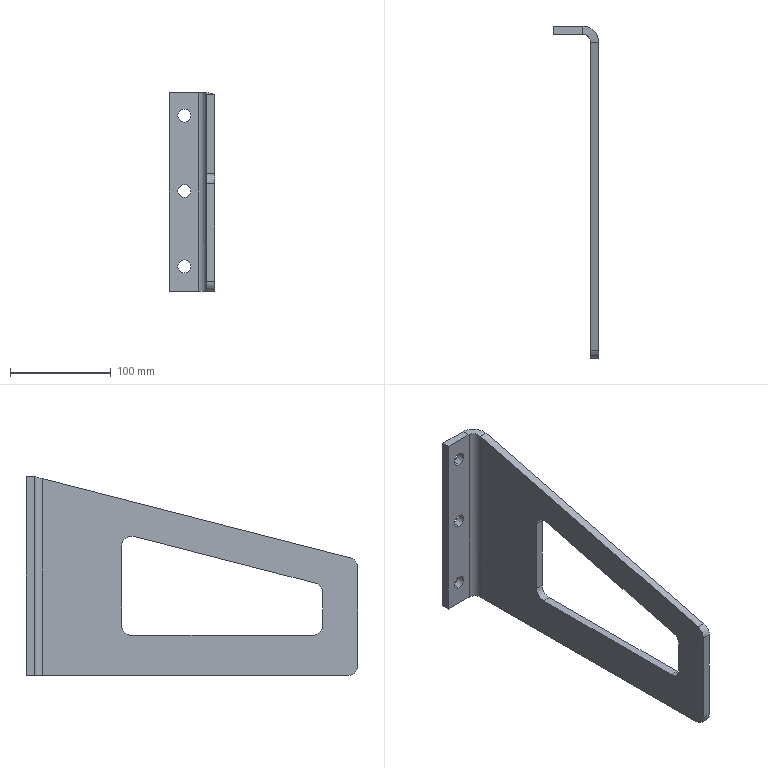Part | SolidWorks | features ICE 2, FlatPattern 1, SMBaseFlange 1, SheetMetal 1 | 1 solid | 30 faces | box 45 x 330 x 197.939 mm | volume 342210 mm3 | plane 15 | cylinder 14 | spline 1 | commonest cylinder face diameters 13 x6 20 x6 16 x1 32 x1
STEP:
#1=CARTESIAN_POINT('',(26.655,269.085,-181.5));
#2=VERTEX_POINT('',#1);
#3=CARTESIAN_POINT('',(26.655,269.085,-168.5));
#4=VERTEX_POINT('',#3);
#5=CARTESIAN_POINT('',(26.655,269.085,-175.));
#6=DIRECTION('',(0.,1.,0.));
#7=DIRECTION('',(0.,0.,1.));
#8=AXIS2_PLACEMENT_3D('',#5,#6,#7);
#9=CIRCLE('',#8,6.5);
#10=EDGE_CURVE('',#2,#4,#9,.T.);
#11=ORIENTED_EDGE('',*,*,#10,.F.);
#12=CARTESIAN_POINT('',(26.655,277.085,-181.5));
#13=VERTEX_POINT('',#12);
#14=CARTESIAN_POINT('',(26.655,-52.915,-181.5));
#15=DIRECTION('',(0.,1.,0.));
#16=VECTOR('',#15,1000.);
#17=LINE('',#14,#16);
#18=EDGE_CURVE('',#2,#13,#17,.T.);
#19=ORIENTED_EDGE('',*,*,#18,.T.);
#20=CARTESIAN_POINT('',(26.655,277.085,-168.5));
#21=VERTEX_POINT('',#20);
#22=CARTESIAN_POINT('',(26.655,277.085,-175.));
#23=DIRECTION('',(0.,1.,0.));
#24=DIRECTION('',(0.,0.,1.));
#25=AXIS2_PLACEMENT_3D('',#22,#23,#24);
#26=CIRCLE('',#25,6.5);
#27=EDGE_CURVE('',#13,#21,#26,.T.);
#28=ORIENTED_EDGE('',*,*,#27,.T.);
#29=CARTESIAN_POINT('',(26.655,-52.915,-168.5));
#30=DIRECTION('',(0.,1.,0.));
#31=VECTOR('',#30,1000.);
#32=LINE('',#29,#31);
#33=EDGE_CURVE('',#4,#21,#32,.T.);
#34=ORIENTED_EDGE('',*,*,#33,.F.);
#35=EDGE_LOOP('',(#11,#19,#28,#34));
#36=FACE_OUTER_BOUND('',#35,.T.);
#37=CARTESIAN_POINT('',(26.655,-52.915,-175.));
#38=DIRECTION('',(0.,1.,0.));
#39=DIRECTION('',(0.,0.,1.));
#40=AXIS2_PLACEMENT_3D('',#37,#38,#39);
#41=CYLINDRICAL_SURFACE('',#40,6.5);
#42=ADVANCED_FACE('',(#36),#41,.F.);
#43=CARTESIAN_POINT('',(26.655,269.085,-106.5));
#44=VERTEX_POINT('',#43);
#45=CARTESIAN_POINT('',(26.655,269.085,-93.5));
#46=VERTEX_POINT('',#45);
#47=CARTESIAN_POINT('',(26.655,269.085,-100.));
#48=DIRECTION('',(0.,1.,0.));
#49=DIRECTION('',(0.,0.,1.));
#50=AXIS2_PLACEMENT_3D('',#47,#48,#49);
#51=CIRCLE('',#50,6.5);
#52=EDGE_CURVE('',#44,#46,#51,.T.);
#53=ORIENTED_EDGE('',*,*,#52,.F.);
#54=CARTESIAN_POINT('',(26.655,277.085,-106.5));
#55=VERTEX_POINT('',#54);
#56=CARTESIAN_POINT('',(26.655,-52.915,-106.5));
#57=DIRECTION('',(0.,1.,0.));
#58=VECTOR('',#57,1000.);
#59=LINE('',#56,#58);
#60=EDGE_CURVE('',#44,#55,#59,.T.);
#61=ORIENTED_EDGE('',*,*,#60,.T.);
#62=CARTESIAN_POINT('',(26.655,277.085,-93.5));
#63=VERTEX_POINT('',#62);
#64=CARTESIAN_POINT('',(26.655,277.085,-100.));
#65=DIRECTION('',(0.,1.,0.));
#66=DIRECTION('',(0.,0.,1.));
#67=AXIS2_PLACEMENT_3D('',#64,#65,#66);
#68=CIRCLE('',#67,6.5);
#69=EDGE_CURVE('',#55,#63,#68,.T.);
#70=ORIENTED_EDGE('',*,*,#69,.T.);
#71=CARTESIAN_POINT('',(26.655,-52.915,-93.5));
#72=DIRECTION('',(0.,1.,0.));
#73=VECTOR('',#72,1000.);
#74=LINE('',#71,#73);
#75=EDGE_CURVE('',#46,#63,#74,.T.);
#76=ORIENTED_EDGE('',*,*,#75,.F.);
#77=EDGE_LOOP('',(#53,#61,#70,#76));
#78=FACE_OUTER_BOUND('',#77,.T.);
#79=CARTESIAN_POINT('',(26.655,-52.915,-100.));
#80=DIRECTION('',(0.,1.,0.));
#81=DIRECTION('',(0.,0.,1.));
#82=AXIS2_PLACEMENT_3D('',#79,#80,#81);
#83=CYLINDRICAL_SURFACE('',#82,6.5);
#84=ADVANCED_FACE('',(#78),#83,.F.);
#85=CARTESIAN_POINT('',(26.655,269.085,-31.5));
#86=VERTEX_POINT('',#85);
#87=CARTESIAN_POINT('',(26.655,269.085,-18.5));
#88=VERTEX_POINT('',#87);
#89=CARTESIAN_POINT('',(26.655,269.085,-25.));
#90=DIRECTION('',(0.,1.,0.));
#91=DIRECTION('',(0.,0.,1.));
#92=AXIS2_PLACEMENT_3D('',#89,#90,#91);
#93=CIRCLE('',#92,6.5);
#94=EDGE_CURVE('',#86,#88,#93,.T.);
#95=ORIENTED_EDGE('',*,*,#94,.F.);
#96=CARTESIAN_POINT('',(26.655,277.085,-31.5));
#97=VERTEX_POINT('',#96);
#98=CARTESIAN_POINT('',(26.655,-52.915,-31.5));
#99=DIRECTION('',(0.,1.,0.));
#100=VECTOR('',#99,1000.);
#101=LINE('',#98,#100);
#102=EDGE_CURVE('',#86,#97,#101,.T.);
#103=ORIENTED_EDGE('',*,*,#102,.T.);
#104=CARTESIAN_POINT('',(26.655,277.085,-18.5));
#105=VERTEX_POINT('',#104);
#106=CARTESIAN_POINT('',(26.655,277.085,-25.));
#107=DIRECTION('',(0.,1.,0.));
#108=DIRECTION('',(0.,0.,1.));
#109=AXIS2_PLACEMENT_3D('',#106,#107,#108);
#110=CIRCLE('',#109,6.5);
#111=EDGE_CURVE('',#97,#105,#110,.T.);
#112=ORIENTED_EDGE('',*,*,#111,.T.);
#113=CARTESIAN_POINT('',(26.655,-52.915,-18.5));
#114=DIRECTION('',(0.,1.,0.));
#115=VECTOR('',#114,1000.);
#116=LINE('',#113,#115);
#117=EDGE_CURVE('',#88,#105,#116,.T.);
#118=ORIENTED_EDGE('',*,*,#117,.F.);
#119=EDGE_LOOP('',(#95,#103,#112,#118));
#120=FACE_OUTER_BOUND('',#119,.T.);
#121=CARTESIAN_POINT('',(26.655,-52.915,-25.));
#122=DIRECTION('',(0.,1.,0.));
#123=DIRECTION('',(0.,0.,1.));
#124=AXIS2_PLACEMENT_3D('',#121,#122,#123);
#125=CYLINDRICAL_SURFACE('',#124,6.5);
#126=ADVANCED_FACE('',(#120),#125,.F.);
#127=CARTESIAN_POINT('',(56.655,-7.915,-160.));
#128=VERTEX_POINT('',#127);
#129=CARTESIAN_POINT('',(56.655,172.085,-160.));
#130=VERTEX_POINT('',#129);
#131=CARTESIAN_POINT('',(56.655,-52.915,-160.));
#132=DIRECTION('',(0.,1.,0.));
#133=VECTOR('',#132,1000.);
#134=LINE('',#131,#133);
#135=EDGE_CURVE('',#128,#130,#134,.T.);
#136=ORIENTED_EDGE('',*,*,#135,.F.);
#137=CARTESIAN_POINT('',(56.655,-17.915,-150.));
#138=VERTEX_POINT('',#137);
#139=CARTESIAN_POINT('',(56.655,-7.915,-150.));
#140=DIRECTION('',(1.,0.,0.));
#141=DIRECTION('',(0.,0.,-1.));
#142=AXIS2_PLACEMENT_3D('',#139,#140,#141);
#143=CIRCLE('',#142,10.);
#144=EDGE_CURVE('',#138,#128,#143,.T.);
#145=ORIENTED_EDGE('',*,*,#144,.F.);
#146=CARTESIAN_POINT('',(56.655,-17.915,-117.751));
#147=VERTEX_POINT('',#146);
#148=CARTESIAN_POINT('',(56.655,-17.915,-200.));
#149=DIRECTION('',(0.,0.,-1.));
#150=VECTOR('',#149,1000.);
#151=LINE('',#148,#150);
#152=EDGE_CURVE('',#147,#138,#151,.T.);
#153=ORIENTED_EDGE('',*,*,#152,.F.);
#154=CARTESIAN_POINT('',(56.655,-10.408,-108.067));
#155=VERTEX_POINT('',#154);
#156=CARTESIAN_POINT('',(56.655,-7.915,-117.751));
#157=DIRECTION('',(1.,0.,0.));
#158=DIRECTION('',(0.,0.,-1.));
#159=AXIS2_PLACEMENT_3D('',#156,#157,#158);
#160=CIRCLE('',#159,10.);
#161=EDGE_CURVE('',#155,#147,#160,.T.);
#162=ORIENTED_EDGE('',*,*,#161,.F.);
#163=CARTESIAN_POINT('',(56.655,169.592,-61.717));
#164=VERTEX_POINT('',#163);
#165=CARTESIAN_POINT('',(56.655,-72.472,-124.049));
#166=DIRECTION('',(0.,-0.9684,-0.2494));
#167=VECTOR('',#166,1000.);
#168=LINE('',#165,#167);
#169=EDGE_CURVE('',#164,#155,#168,.T.);
#170=ORIENTED_EDGE('',*,*,#169,.F.);
#171=CARTESIAN_POINT('',(56.655,182.085,-71.401));
#172=VERTEX_POINT('',#171);
#173=CARTESIAN_POINT('',(56.655,172.085,-71.401));
#174=DIRECTION('',(1.,0.,0.));
#175=DIRECTION('',(0.,0.,-1.));
#176=AXIS2_PLACEMENT_3D('',#173,#174,#175);
#177=CIRCLE('',#176,10.);
#178=EDGE_CURVE('',#172,#164,#177,.T.);
#179=ORIENTED_EDGE('',*,*,#178,.F.);
#180=CARTESIAN_POINT('',(56.655,182.085,-150.));
#181=VERTEX_POINT('',#180);
#182=CARTESIAN_POINT('',(56.655,182.085,-200.));
#183=DIRECTION('',(0.,0.,1.));
#184=VECTOR('',#183,1000.);
#185=LINE('',#182,#184);
#186=EDGE_CURVE('',#181,#172,#185,.T.);
#187=ORIENTED_EDGE('',*,*,#186,.F.);
#188=CARTESIAN_POINT('',(56.655,172.085,-150.));
#189=DIRECTION('',(1.,0.,0.));
#190=DIRECTION('',(0.,0.,-1.));
#191=AXIS2_PLACEMENT_3D('',#188,#189,#190);
#192=CIRCLE('',#191,10.);
#193=EDGE_CURVE('',#130,#181,#192,.T.);
#194=ORIENTED_EDGE('',*,*,#193,.F.);
#195=EDGE_LOOP('',(#136,#145,#153,#162,#170,#179,#187,#194));
#196=FACE_BOUND('',#195,.T.);
#197=CARTESIAN_POINT('',(56.655,-45.409,-83.067));
#198=VERTEX_POINT('',#197);
#199=CARTESIAN_POINT('',(56.655,261.085,-4.121));
#200=VERTEX_POINT('',#199);
#201=CARTESIAN_POINT('',(56.655,-45.409,-83.067));
#202=DIRECTION('',(0.,0.9684,0.2494));
#203=VECTOR('',#202,1000.);
#204=LINE('',#201,#203);
#205=EDGE_CURVE('',#198,#200,#204,.T.);
#206=ORIENTED_EDGE('',*,*,#205,.F.);
#207=CARTESIAN_POINT('',(56.655,-52.915,-92.751));
#208=VERTEX_POINT('',#207);
#209=CARTESIAN_POINT('',(56.655,-42.915,-92.751));
#210=DIRECTION('',(-1.,0.,0.));
#211=DIRECTION('',(0.,0.,1.));
#212=AXIS2_PLACEMENT_3D('',#209,#210,#211);
#213=CIRCLE('',#212,10.);
#214=EDGE_CURVE('',#208,#198,#213,.T.);
#215=ORIENTED_EDGE('',*,*,#214,.F.);
#216=CARTESIAN_POINT('',(56.655,-52.915,-190.));
#217=VERTEX_POINT('',#216);
#218=CARTESIAN_POINT('',(56.655,-52.915,-200.));
#219=DIRECTION('',(0.,0.,1.));
#220=VECTOR('',#219,1000.);
#221=LINE('',#218,#220);
#222=EDGE_CURVE('',#217,#208,#221,.T.);
#223=ORIENTED_EDGE('',*,*,#222,.F.);
#224=CARTESIAN_POINT('',(56.655,-42.915,-200.));
#225=VERTEX_POINT('',#224);
#226=CARTESIAN_POINT('',(56.655,-42.915,-190.));
#227=DIRECTION('',(-1.,0.,0.));
#228=DIRECTION('',(0.,0.,-1.));
#229=AXIS2_PLACEMENT_3D('',#226,#227,#228);
#230=CIRCLE('',#229,10.);
#231=EDGE_CURVE('',#225,#217,#230,.T.);
#232=ORIENTED_EDGE('',*,*,#231,.F.);
#233=CARTESIAN_POINT('',(56.655,261.085,-200.));
#234=VERTEX_POINT('',#233);
#235=CARTESIAN_POINT('',(56.655,-52.915,-200.));
#236=DIRECTION('',(0.,1.,0.));
#237=VECTOR('',#236,1000.);
#238=LINE('',#235,#237);
#239=EDGE_CURVE('',#225,#234,#238,.T.);
#240=ORIENTED_EDGE('',*,*,#239,.T.);
#241=CARTESIAN_POINT('',(56.655,261.085,-200.));
#242=DIRECTION('',(0.,0.,1.));
#243=VECTOR('',#242,1000.);
#244=LINE('',#241,#243);
#245=EDGE_CURVE('',#234,#200,#244,.T.);
#246=ORIENTED_EDGE('',*,*,#245,.T.);
#247=EDGE_LOOP('',(#206,#215,#223,#232,#240,#246));
#248=FACE_OUTER_BOUND('',#247,.T.);
#249=CARTESIAN_POINT('',(56.655,-52.915,-200.));
#250=DIRECTION('',(1.,0.,0.));
#251=DIRECTION('',(0.,0.,-1.));
#252=AXIS2_PLACEMENT_3D('',#249,#250,#251);
#253=PLANE('',#252);
#254=ADVANCED_FACE('',(#196,#248),#253,.T.);
#255=CARTESIAN_POINT('',(48.655,-17.915,-150.));
#256=VERTEX_POINT('',#255);
#257=CARTESIAN_POINT('',(48.655,-7.915,-160.));
#258=VERTEX_POINT('',#257);
#259=CARTESIAN_POINT('',(48.655,-7.915,-150.));
#260=DIRECTION('',(1.,0.,0.));
#261=DIRECTION('',(0.,0.,-1.));
#262=AXIS2_PLACEMENT_3D('',#259,#260,#261);
#263=CIRCLE('',#262,10.);
#264=EDGE_CURVE('',#256,#258,#263,.T.);
#265=ORIENTED_EDGE('',*,*,#264,.T.);
#266=CARTESIAN_POINT('',(48.655,172.085,-160.));
#267=VERTEX_POINT('',#266);
#268=CARTESIAN_POINT('',(48.655,-52.915,-160.));
#269=DIRECTION('',(0.,1.,0.));
#270=VECTOR('',#269,1000.);
#271=LINE('',#268,#270);
#272=EDGE_CURVE('',#258,#267,#271,.T.);
#273=ORIENTED_EDGE('',*,*,#272,.T.);
#274=CARTESIAN_POINT('',(48.655,182.085,-150.));
#275=VERTEX_POINT('',#274);
#276=CARTESIAN_POINT('',(48.655,172.085,-150.));
#277=DIRECTION('',(1.,0.,0.));
#278=DIRECTION('',(0.,0.,-1.));
#279=AXIS2_PLACEMENT_3D('',#276,#277,#278);
#280=CIRCLE('',#279,10.);
#281=EDGE_CURVE('',#267,#275,#280,.T.);
#282=ORIENTED_EDGE('',*,*,#281,.T.);
#283=CARTESIAN_POINT('',(48.655,182.085,-71.401));
#284=VERTEX_POINT('',#283);
#285=CARTESIAN_POINT('',(48.655,182.085,-200.));
#286=DIRECTION('',(0.,0.,1.));
#287=VECTOR('',#286,1000.);
#288=LINE('',#285,#287);
#289=EDGE_CURVE('',#275,#284,#288,.T.);
#290=ORIENTED_EDGE('',*,*,#289,.T.);
#291=CARTESIAN_POINT('',(48.655,169.592,-61.717));
#292=VERTEX_POINT('',#291);
#293=CARTESIAN_POINT('',(48.655,172.085,-71.401));
#294=DIRECTION('',(1.,0.,0.));
#295=DIRECTION('',(0.,0.,-1.));
#296=AXIS2_PLACEMENT_3D('',#293,#294,#295);
#297=CIRCLE('',#296,10.);
#298=EDGE_CURVE('',#284,#292,#297,.T.);
#299=ORIENTED_EDGE('',*,*,#298,.T.);
#300=CARTESIAN_POINT('',(48.655,-10.408,-108.067));
#301=VERTEX_POINT('',#300);
#302=CARTESIAN_POINT('',(48.655,-72.472,-124.049));
#303=DIRECTION('',(0.,-0.9684,-0.2494));
#304=VECTOR('',#303,1000.);
#305=LINE('',#302,#304);
#306=EDGE_CURVE('',#292,#301,#305,.T.);
#307=ORIENTED_EDGE('',*,*,#306,.T.);
#308=CARTESIAN_POINT('',(48.655,-17.915,-117.751));
#309=VERTEX_POINT('',#308);
#310=CARTESIAN_POINT('',(48.655,-7.915,-117.751));
#311=DIRECTION('',(1.,0.,0.));
#312=DIRECTION('',(0.,0.,-1.));
#313=AXIS2_PLACEMENT_3D('',#310,#311,#312);
#314=CIRCLE('',#313,10.);
#315=EDGE_CURVE('',#301,#309,#314,.T.);
#316=ORIENTED_EDGE('',*,*,#315,.T.);
#317=CARTESIAN_POINT('',(48.655,-17.915,-200.));
#318=DIRECTION('',(0.,0.,-1.));
#319=VECTOR('',#318,1000.);
#320=LINE('',#317,#319);
#321=EDGE_CURVE('',#309,#256,#320,.T.);
#322=ORIENTED_EDGE('',*,*,#321,.T.);
#323=EDGE_LOOP('',(#265,#273,#282,#290,#299,#307,#316,#322));
#324=FACE_BOUND('',#323,.T.);
#325=CARTESIAN_POINT('',(48.655,-52.915,-92.751));
#326=VERTEX_POINT('',#325);
#327=CARTESIAN_POINT('',(48.655,-45.409,-83.067));
#328=VERTEX_POINT('',#327);
#329=CARTESIAN_POINT('',(48.655,-42.915,-92.751));
#330=DIRECTION('',(-1.,0.,0.));
#331=DIRECTION('',(0.,0.,1.));
#332=AXIS2_PLACEMENT_3D('',#329,#330,#331);
#333=CIRCLE('',#332,10.);
#334=EDGE_CURVE('',#326,#328,#333,.T.);
#335=ORIENTED_EDGE('',*,*,#334,.T.);
#336=CARTESIAN_POINT('',(48.655,261.085,-4.121));
#337=VERTEX_POINT('',#336);
#338=CARTESIAN_POINT('',(48.655,-45.409,-83.067));
#339=DIRECTION('',(0.,0.9684,0.2494));
#340=VECTOR('',#339,1000.);
#341=LINE('',#338,#340);
#342=EDGE_CURVE('',#328,#337,#341,.T.);
#343=ORIENTED_EDGE('',*,*,#342,.T.);
#344=CARTESIAN_POINT('',(48.655,261.085,-200.));
#345=VERTEX_POINT('',#344);
#346=CARTESIAN_POINT('',(48.655,261.085,-200.));
#347=DIRECTION('',(0.,0.,1.));
#348=VECTOR('',#347,1000.);
#349=LINE('',#346,#348);
#350=EDGE_CURVE('',#345,#337,#349,.T.);
#351=ORIENTED_EDGE('',*,*,#350,.F.);
#352=CARTESIAN_POINT('',(48.655,-42.915,-200.));
#353=VERTEX_POINT('',#352);
#354=CARTESIAN_POINT('',(48.655,-52.915,-200.));
#355=DIRECTION('',(0.,1.,0.));
#356=VECTOR('',#355,1000.);
#357=LINE('',#354,#356);
#358=EDGE_CURVE('',#353,#345,#357,.T.);
#359=ORIENTED_EDGE('',*,*,#358,.F.);
#360=CARTESIAN_POINT('',(48.655,-52.915,-190.));
#361=VERTEX_POINT('',#360);
#362=CARTESIAN_POINT('',(48.655,-42.915,-190.));
#363=DIRECTION('',(-1.,0.,0.));
#364=DIRECTION('',(0.,0.,-1.));
#365=AXIS2_PLACEMENT_3D('',#362,#363,#364);
#366=CIRCLE('',#365,10.);
#367=EDGE_CURVE('',#353,#361,#366,.T.);
#368=ORIENTED_EDGE('',*,*,#367,.T.);
#369=CARTESIAN_POINT('',(48.655,-52.915,-200.));
#370=DIRECTION('',(0.,0.,1.));
#371=VECTOR('',#370,1000.);
#372=LINE('',#369,#371);
#373=EDGE_CURVE('',#361,#326,#372,.T.);
#374=ORIENTED_EDGE('',*,*,#373,.T.);
#375=EDGE_LOOP('',(#335,#343,#351,#359,#368,#374));
#376=FACE_OUTER_BOUND('',#375,.T.);
#377=CARTESIAN_POINT('',(48.655,-52.915,-200.));
#378=DIRECTION('',(1.,0.,0.));
#379=DIRECTION('',(0.,0.,-1.));
#380=AXIS2_PLACEMENT_3D('',#377,#378,#379);
#381=PLANE('',#380);
#382=ADVANCED_FACE('',(#324,#376),#381,.F.);
#383=CARTESIAN_POINT('',(26.655,277.085,-175.));
#384=DIRECTION('',(0.,1.,0.));
#385=DIRECTION('',(0.,0.,1.));
#386=AXIS2_PLACEMENT_3D('',#383,#384,#385);
#387=CIRCLE('',#386,6.5);
#388=EDGE_CURVE('',#21,#13,#387,.T.);
#389=ORIENTED_EDGE('',*,*,#388,.F.);
#390=ORIENTED_EDGE('',*,*,#27,.F.);
#391=EDGE_LOOP('',(#389,#390));
#392=FACE_BOUND('',#391,.T.);
#393=CARTESIAN_POINT('',(26.655,277.085,-100.));
#394=DIRECTION('',(0.,1.,0.));
#395=DIRECTION('',(0.,0.,1.));
#396=AXIS2_PLACEMENT_3D('',#393,#394,#395);
#397=CIRCLE('',#396,6.5);
#398=EDGE_CURVE('',#63,#55,#397,.T.);
#399=ORIENTED_EDGE('',*,*,#398,.F.);
#400=ORIENTED_EDGE('',*,*,#69,.F.);
#401=EDGE_LOOP('',(#399,#400));
#402=FACE_BOUND('',#401,.T.);
#403=CARTESIAN_POINT('',(26.655,277.085,-25.));
#404=DIRECTION('',(0.,1.,0.));
#405=DIRECTION('',(0.,0.,1.));
#406=AXIS2_PLACEMENT_3D('',#403,#404,#405);
#407=CIRCLE('',#406,6.5);
#408=EDGE_CURVE('',#105,#97,#407,.T.);
#409=ORIENTED_EDGE('',*,*,#408,.F.);
#410=ORIENTED_EDGE('',*,*,#111,.F.);
#411=EDGE_LOOP('',(#409,#410));
#412=FACE_BOUND('',#411,.T.);
#413=CARTESIAN_POINT('',(11.655,277.085,-200.));
#414=VERTEX_POINT('',#413);
#415=CARTESIAN_POINT('',(11.655,277.085,-2.061));
#416=VERTEX_POINT('',#415);
#417=CARTESIAN_POINT('',(11.655,277.085,-200.));
#418=DIRECTION('',(0.,0.,1.));
#419=VECTOR('',#418,1000.);
#420=LINE('',#417,#419);
#421=EDGE_CURVE('',#414,#416,#420,.T.);
#422=ORIENTED_EDGE('',*,*,#421,.T.);
#423=CARTESIAN_POINT('',(40.655,277.085,-2.061));
#424=VERTEX_POINT('',#423);
#425=CARTESIAN_POINT('',(48.655,277.085,-2.061));
#426=DIRECTION('',(-1.,0.,0.));
#427=VECTOR('',#426,1000.);
#428=LINE('',#425,#427);
#429=EDGE_CURVE('',#424,#416,#428,.T.);
#430=ORIENTED_EDGE('',*,*,#429,.F.);
#431=CARTESIAN_POINT('',(40.655,277.085,-200.));
#432=VERTEX_POINT('',#431);
#433=CARTESIAN_POINT('',(40.655,277.085,-200.));
#434=DIRECTION('',(0.,0.,1.));
#435=VECTOR('',#434,1000.);
#436=LINE('',#433,#435);
#437=EDGE_CURVE('',#432,#424,#436,.T.);
#438=ORIENTED_EDGE('',*,*,#437,.F.);
#439=CARTESIAN_POINT('',(48.655,277.085,-200.));
#440=DIRECTION('',(-1.,0.,0.));
#441=VECTOR('',#440,1000.);
#442=LINE('',#439,#441);
#443=EDGE_CURVE('',#432,#414,#442,.T.);
#444=ORIENTED_EDGE('',*,*,#443,.T.);
#445=EDGE_LOOP('',(#422,#430,#438,#444));
#446=FACE_OUTER_BOUND('',#445,.T.);
#447=CARTESIAN_POINT('',(48.655,277.085,-200.));
#448=DIRECTION('',(0.,1.,0.));
#449=DIRECTION('',(0.,0.,1.));
#450=AXIS2_PLACEMENT_3D('',#447,#448,#449);
#451=PLANE('',#450);
#452=ADVANCED_FACE('',(#392,#402,#412,#446),#451,.T.);
#453=ORIENTED_EDGE('',*,*,#437,.T.);
#454=CARTESIAN_POINT('',(56.655,261.085,-4.121));
#455=CARTESIAN_POINT('',(56.655,270.458,-2.914));
#456=CARTESIAN_POINT('',(50.027,277.085,-2.061));
#457=CARTESIAN_POINT('',(40.655,277.085,-2.061));
#458=(BOUNDED_CURVE()B_SPLINE_CURVE(3,(#454,#455,#456,#457),.UNSPECIFIED.,.F.,.T.)B_SPLINE_CURVE_WITH_KNOTS((4,4),(4.712,6.283),.UNSPECIFIED.)CURVE()GEOMETRIC_REPRESENTATION_ITEM()RATIONAL_B_SPLINE_CURVE((1.,0.8047,0.8047,1.))REPRESENTATION_ITEM(''));
#459=EDGE_CURVE('',#200,#424,#458,.T.);
#460=ORIENTED_EDGE('',*,*,#459,.F.);
#461=ORIENTED_EDGE('',*,*,#245,.F.);
#462=CARTESIAN_POINT('',(40.655,261.085,-200.));
#463=DIRECTION('',(0.,0.,1.));
#464=DIRECTION('',(1.,0.,0.));
#465=AXIS2_PLACEMENT_3D('',#462,#463,#464);
#466=CIRCLE('',#465,16.);
#467=EDGE_CURVE('',#234,#432,#466,.T.);
#468=ORIENTED_EDGE('',*,*,#467,.T.);
#469=EDGE_LOOP('',(#453,#460,#461,#468));
#470=FACE_OUTER_BOUND('',#469,.T.);
#471=CARTESIAN_POINT('',(40.655,261.085,-200.));
#472=DIRECTION('',(0.,0.,1.));
#473=DIRECTION('',(1.,0.,0.));
#474=AXIS2_PLACEMENT_3D('',#471,#472,#473);
#475=CYLINDRICAL_SURFACE('',#474,16.);
#476=ADVANCED_FACE('',(#470),#475,.T.);
#477=CARTESIAN_POINT('',(40.655,269.085,-2.061));
#478=VERTEX_POINT('',#477);
#479=CARTESIAN_POINT('',(48.655,261.085,-4.121));
#480=CARTESIAN_POINT('',(48.655,265.772,-2.914));
#481=CARTESIAN_POINT('',(45.341,269.085,-2.061));
#482=CARTESIAN_POINT('',(40.655,269.085,-2.061));
#483=(BOUNDED_CURVE()B_SPLINE_CURVE(3,(#479,#480,#481,#482),.UNSPECIFIED.,.F.,.T.)B_SPLINE_CURVE_WITH_KNOTS((4,4),(4.712,6.283),.UNSPECIFIED.)CURVE()GEOMETRIC_REPRESENTATION_ITEM()RATIONAL_B_SPLINE_CURVE((1.,0.8047,0.8047,1.))REPRESENTATION_ITEM(''));
#484=EDGE_CURVE('',#337,#478,#483,.T.);
#485=ORIENTED_EDGE('',*,*,#484,.T.);
#486=CARTESIAN_POINT('',(40.655,269.085,-200.));
#487=VERTEX_POINT('',#486);
#488=CARTESIAN_POINT('',(40.655,269.085,-200.));
#489=DIRECTION('',(0.,0.,1.));
#490=VECTOR('',#489,1000.);
#491=LINE('',#488,#490);
#492=EDGE_CURVE('',#487,#478,#491,.T.);
#493=ORIENTED_EDGE('',*,*,#492,.F.);
#494=CARTESIAN_POINT('',(40.655,261.085,-200.));
#495=DIRECTION('',(0.,0.,1.));
#496=DIRECTION('',(-1.,0.,0.));
#497=AXIS2_PLACEMENT_3D('',#494,#495,#496);
#498=CIRCLE('',#497,8.);
#499=EDGE_CURVE('',#345,#487,#498,.T.);
#500=ORIENTED_EDGE('',*,*,#499,.F.);
#501=ORIENTED_EDGE('',*,*,#350,.T.);
#502=EDGE_LOOP('',(#485,#493,#500,#501));
#503=FACE_OUTER_BOUND('',#502,.T.);
#504=CARTESIAN_POINT('',(40.655,261.085,-200.));
#505=DIRECTION('',(0.,0.,1.));
#506=DIRECTION('',(1.,0.,0.));
#507=AXIS2_PLACEMENT_3D('',#504,#505,#506);
#508=CYLINDRICAL_SURFACE('',#507,8.);
#509=ADVANCED_FACE('',(#503),#508,.F.);
#510=CARTESIAN_POINT('',(26.655,269.085,-175.));
#511=DIRECTION('',(0.,1.,0.));
#512=DIRECTION('',(0.,0.,1.));
#513=AXIS2_PLACEMENT_3D('',#510,#511,#512);
#514=CIRCLE('',#513,6.5);
#515=EDGE_CURVE('',#4,#2,#514,.T.);
#516=ORIENTED_EDGE('',*,*,#515,.T.);
#517=ORIENTED_EDGE('',*,*,#10,.T.);
#518=EDGE_LOOP('',(#516,#517));
#519=FACE_BOUND('',#518,.T.);
#520=CARTESIAN_POINT('',(26.655,269.085,-100.));
#521=DIRECTION('',(0.,1.,0.));
#522=DIRECTION('',(0.,0.,1.));
#523=AXIS2_PLACEMENT_3D('',#520,#521,#522);
#524=CIRCLE('',#523,6.5);
#525=EDGE_CURVE('',#46,#44,#524,.T.);
#526=ORIENTED_EDGE('',*,*,#525,.T.);
#527=ORIENTED_EDGE('',*,*,#52,.T.);
#528=EDGE_LOOP('',(#526,#527));
#529=FACE_BOUND('',#528,.T.);
#530=CARTESIAN_POINT('',(26.655,269.085,-25.));
#531=DIRECTION('',(0.,1.,0.));
#532=DIRECTION('',(0.,0.,1.));
#533=AXIS2_PLACEMENT_3D('',#530,#531,#532);
#534=CIRCLE('',#533,6.5);
#535=EDGE_CURVE('',#88,#86,#534,.T.);
#536=ORIENTED_EDGE('',*,*,#535,.T.);
#537=ORIENTED_EDGE('',*,*,#94,.T.);
#538=EDGE_LOOP('',(#536,#537));
#539=FACE_BOUND('',#538,.T.);
#540=CARTESIAN_POINT('',(11.655,269.085,-2.061));
#541=VERTEX_POINT('',#540);
#542=CARTESIAN_POINT('',(48.655,269.085,-2.061));
#543=DIRECTION('',(-1.,0.,0.));
#544=VECTOR('',#543,1000.);
#545=LINE('',#542,#544);
#546=EDGE_CURVE('',#478,#541,#545,.T.);
#547=ORIENTED_EDGE('',*,*,#546,.T.);
#548=CARTESIAN_POINT('',(11.655,269.085,-200.));
#549=VERTEX_POINT('',#548);
#550=CARTESIAN_POINT('',(11.655,269.085,-200.));
#551=DIRECTION('',(0.,0.,1.));
#552=VECTOR('',#551,1000.);
#553=LINE('',#550,#552);
#554=EDGE_CURVE('',#549,#541,#553,.T.);
#555=ORIENTED_EDGE('',*,*,#554,.F.);
#556=CARTESIAN_POINT('',(48.655,269.085,-200.));
#557=DIRECTION('',(-1.,0.,0.));
#558=VECTOR('',#557,1000.);
#559=LINE('',#556,#558);
#560=EDGE_CURVE('',#487,#549,#559,.T.);
#561=ORIENTED_EDGE('',*,*,#560,.F.);
#562=ORIENTED_EDGE('',*,*,#492,.T.);
#563=EDGE_LOOP('',(#547,#555,#561,#562));
#564=FACE_OUTER_BOUND('',#563,.T.);
#565=CARTESIAN_POINT('',(48.655,269.085,-200.));
#566=DIRECTION('',(0.,1.,0.));
#567=DIRECTION('',(0.,0.,1.));
#568=AXIS2_PLACEMENT_3D('',#565,#566,#567);
#569=PLANE('',#568);
#570=ADVANCED_FACE('',(#519,#529,#539,#564),#569,.F.);
#571=CARTESIAN_POINT('',(11.655,269.085,-2.061));
#572=DIRECTION('',(0.,1.,0.));
#573=VECTOR('',#572,1000.);
#574=LINE('',#571,#573);
#575=EDGE_CURVE('',#541,#416,#574,.T.);
#576=ORIENTED_EDGE('',*,*,#575,.T.);
#577=ORIENTED_EDGE('',*,*,#421,.F.);
#578=CARTESIAN_POINT('',(11.655,269.085,-200.));
#579=DIRECTION('',(0.,1.,0.));
#580=VECTOR('',#579,1000.);
#581=LINE('',#578,#580);
#582=EDGE_CURVE('',#549,#414,#581,.T.);
#583=ORIENTED_EDGE('',*,*,#582,.F.);
#584=ORIENTED_EDGE('',*,*,#554,.T.);
#585=EDGE_LOOP('',(#576,#577,#583,#584));
#586=FACE_OUTER_BOUND('',#585,.T.);
#587=CARTESIAN_POINT('',(11.655,269.085,-200.));
#588=DIRECTION('',(1.,0.,0.));
#589=DIRECTION('',(0.,0.,-1.));
#590=AXIS2_PLACEMENT_3D('',#587,#588,#589);
#591=PLANE('',#590);
#592=ADVANCED_FACE('',(#586),#591,.F.);
#593=CARTESIAN_POINT('',(48.655,261.085,-200.));
#594=DIRECTION('',(1.,0.,0.));
#595=VECTOR('',#594,1000.);
#596=LINE('',#593,#595);
#597=EDGE_CURVE('',#345,#234,#596,.T.);
#598=ORIENTED_EDGE('',*,*,#597,.F.);
#599=ORIENTED_EDGE('',*,*,#499,.T.);
#600=CARTESIAN_POINT('',(40.655,277.085,-200.));
#601=DIRECTION('',(0.,-1.,0.));
#602=VECTOR('',#601,1000.);
#603=LINE('',#600,#602);
#604=EDGE_CURVE('',#432,#487,#603,.T.);
#605=ORIENTED_EDGE('',*,*,#604,.F.);
#606=ORIENTED_EDGE('',*,*,#467,.F.);
#607=EDGE_LOOP('',(#598,#599,#605,#606));
#608=FACE_OUTER_BOUND('',#607,.T.);
#609=CARTESIAN_POINT('',(48.655,261.085,-200.));
#610=DIRECTION('',(0.,0.,-1.));
#611=DIRECTION('',(-1.,0.,0.));
#612=AXIS2_PLACEMENT_3D('',#609,#610,#611);
#613=PLANE('',#612);
#614=ADVANCED_FACE('',(#608),#613,.T.);
#615=CARTESIAN_POINT('',(48.655,-42.915,-200.));
#616=DIRECTION('',(1.,0.,0.));
#617=VECTOR('',#616,1000.);
#618=LINE('',#615,#617);
#619=EDGE_CURVE('',#353,#225,#618,.T.);
#620=ORIENTED_EDGE('',*,*,#619,.F.);
#621=ORIENTED_EDGE('',*,*,#358,.T.);
#622=ORIENTED_EDGE('',*,*,#597,.T.);
#623=ORIENTED_EDGE('',*,*,#239,.F.);
#624=EDGE_LOOP('',(#620,#621,#622,#623));
#625=FACE_OUTER_BOUND('',#624,.T.);
#626=CARTESIAN_POINT('',(40.655,277.085,-200.));
#627=DIRECTION('',(0.,0.,-1.));
#628=DIRECTION('',(-1.,0.,0.));
#629=AXIS2_PLACEMENT_3D('',#626,#627,#628);
#630=PLANE('',#629);
#631=ADVANCED_FACE('',(#625),#630,.T.);
#632=ORIENTED_EDGE('',*,*,#222,.T.);
#633=CARTESIAN_POINT('',(56.655,-52.915,-92.751));
#634=DIRECTION('',(-1.,0.,0.));
#635=VECTOR('',#634,1000.);
#636=LINE('',#633,#635);
#637=EDGE_CURVE('',#208,#326,#636,.T.);
#638=ORIENTED_EDGE('',*,*,#637,.T.);
#639=ORIENTED_EDGE('',*,*,#373,.F.);
#640=CARTESIAN_POINT('',(48.655,-52.915,-190.));
#641=DIRECTION('',(1.,0.,0.));
#642=VECTOR('',#641,1000.);
#643=LINE('',#640,#642);
#644=EDGE_CURVE('',#361,#217,#643,.T.);
#645=ORIENTED_EDGE('',*,*,#644,.T.);
#646=EDGE_LOOP('',(#632,#638,#639,#645));
#647=FACE_OUTER_BOUND('',#646,.T.);
#648=CARTESIAN_POINT('',(56.655,-52.915,-200.));
#649=DIRECTION('',(0.,1.,0.));
#650=DIRECTION('',(0.,0.,1.));
#651=AXIS2_PLACEMENT_3D('',#648,#649,#650);
#652=PLANE('',#651);
#653=ADVANCED_FACE('',(#647),#652,.F.);
#654=ORIENTED_EDGE('',*,*,#443,.F.);
#655=ORIENTED_EDGE('',*,*,#604,.T.);
#656=ORIENTED_EDGE('',*,*,#560,.T.);
#657=ORIENTED_EDGE('',*,*,#582,.T.);
#658=EDGE_LOOP('',(#654,#655,#656,#657));
#659=FACE_OUTER_BOUND('',#658,.T.);
#660=CARTESIAN_POINT('',(40.655,261.085,-200.));
#661=DIRECTION('',(0.,0.,-1.));
#662=DIRECTION('',(-1.,0.,0.));
#663=AXIS2_PLACEMENT_3D('',#660,#661,#662);
#664=PLANE('',#663);
#665=ADVANCED_FACE('',(#659),#664,.T.);
#666=ORIENTED_EDGE('',*,*,#644,.F.);
#667=ORIENTED_EDGE('',*,*,#367,.F.);
#668=ORIENTED_EDGE('',*,*,#619,.T.);
#669=ORIENTED_EDGE('',*,*,#231,.T.);
#670=EDGE_LOOP('',(#666,#667,#668,#669));
#671=FACE_OUTER_BOUND('',#670,.T.);
#672=CARTESIAN_POINT('',(48.655,-42.915,-190.));
#673=DIRECTION('',(1.,0.,0.));
#674=DIRECTION('',(0.,0.,-1.));
#675=AXIS2_PLACEMENT_3D('',#672,#673,#674);
#676=CYLINDRICAL_SURFACE('',#675,10.);
#677=ADVANCED_FACE('',(#671),#676,.T.);
#678=CARTESIAN_POINT('',(48.655,-7.915,-160.));
#679=DIRECTION('',(1.,0.,0.));
#680=VECTOR('',#679,1000.);
#681=LINE('',#678,#680);
#682=EDGE_CURVE('',#258,#128,#681,.T.);
#683=ORIENTED_EDGE('',*,*,#682,.F.);
#684=ORIENTED_EDGE('',*,*,#264,.F.);
#685=CARTESIAN_POINT('',(48.655,-17.915,-150.));
#686=DIRECTION('',(1.,0.,0.));
#687=VECTOR('',#686,1000.);
#688=LINE('',#685,#687);
#689=EDGE_CURVE('',#256,#138,#688,.T.);
#690=ORIENTED_EDGE('',*,*,#689,.T.);
#691=ORIENTED_EDGE('',*,*,#144,.T.);
#692=EDGE_LOOP('',(#683,#684,#690,#691));
#693=FACE_OUTER_BOUND('',#692,.T.);
#694=CARTESIAN_POINT('',(48.655,-7.915,-150.));
#695=DIRECTION('',(1.,0.,0.));
#696=DIRECTION('',(0.,0.,-1.));
#697=AXIS2_PLACEMENT_3D('',#694,#695,#696);
#698=CYLINDRICAL_SURFACE('',#697,10.);
#699=ADVANCED_FACE('',(#693),#698,.F.);
#700=ORIENTED_EDGE('',*,*,#689,.F.);
#701=ORIENTED_EDGE('',*,*,#321,.F.);
#702=CARTESIAN_POINT('',(48.655,-17.915,-117.751));
#703=DIRECTION('',(1.,0.,0.));
#704=VECTOR('',#703,1000.);
#705=LINE('',#702,#704);
#706=EDGE_CURVE('',#309,#147,#705,.T.);
#707=ORIENTED_EDGE('',*,*,#706,.T.);
#708=ORIENTED_EDGE('',*,*,#152,.T.);
#709=EDGE_LOOP('',(#700,#701,#707,#708));
#710=FACE_OUTER_BOUND('',#709,.T.);
#711=CARTESIAN_POINT('',(48.655,-17.915,-200.));
#712=DIRECTION('',(0.,-1.,0.));
#713=DIRECTION('',(0.,0.,-1.));
#714=AXIS2_PLACEMENT_3D('',#711,#712,#713);
#715=PLANE('',#714);
#716=ADVANCED_FACE('',(#710),#715,.F.);
#717=ORIENTED_EDGE('',*,*,#706,.F.);
#718=ORIENTED_EDGE('',*,*,#315,.F.);
#719=CARTESIAN_POINT('',(48.655,-10.408,-108.067));
#720=DIRECTION('',(1.,0.,0.));
#721=VECTOR('',#720,1000.);
#722=LINE('',#719,#721);
#723=EDGE_CURVE('',#301,#155,#722,.T.);
#724=ORIENTED_EDGE('',*,*,#723,.T.);
#725=ORIENTED_EDGE('',*,*,#161,.T.);
#726=EDGE_LOOP('',(#717,#718,#724,#725));
#727=FACE_OUTER_BOUND('',#726,.T.);
#728=CARTESIAN_POINT('',(48.655,-7.915,-117.751));
#729=DIRECTION('',(1.,0.,0.));
#730=DIRECTION('',(0.,0.,-1.));
#731=AXIS2_PLACEMENT_3D('',#728,#729,#730);
#732=CYLINDRICAL_SURFACE('',#731,10.);
#733=ADVANCED_FACE('',(#727),#732,.F.);
#734=ORIENTED_EDGE('',*,*,#723,.F.);
#735=ORIENTED_EDGE('',*,*,#306,.F.);
#736=CARTESIAN_POINT('',(48.655,169.592,-61.717));
#737=DIRECTION('',(1.,0.,0.));
#738=VECTOR('',#737,1000.);
#739=LINE('',#736,#738);
#740=EDGE_CURVE('',#292,#164,#739,.T.);
#741=ORIENTED_EDGE('',*,*,#740,.T.);
#742=ORIENTED_EDGE('',*,*,#169,.T.);
#743=EDGE_LOOP('',(#734,#735,#741,#742));
#744=FACE_OUTER_BOUND('',#743,.T.);
#745=CARTESIAN_POINT('',(48.655,-72.472,-124.049));
#746=DIRECTION('',(0.,-0.2494,0.9684));
#747=DIRECTION('',(0.,-0.9684,-0.2494));
#748=AXIS2_PLACEMENT_3D('',#745,#746,#747);
#749=PLANE('',#748);
#750=ADVANCED_FACE('',(#744),#749,.F.);
#751=ORIENTED_EDGE('',*,*,#740,.F.);
#752=ORIENTED_EDGE('',*,*,#298,.F.);
#753=CARTESIAN_POINT('',(48.655,182.085,-71.401));
#754=DIRECTION('',(1.,0.,0.));
#755=VECTOR('',#754,1000.);
#756=LINE('',#753,#755);
#757=EDGE_CURVE('',#284,#172,#756,.T.);
#758=ORIENTED_EDGE('',*,*,#757,.T.);
#759=ORIENTED_EDGE('',*,*,#178,.T.);
#760=EDGE_LOOP('',(#751,#752,#758,#759));
#761=FACE_OUTER_BOUND('',#760,.T.);
#762=CARTESIAN_POINT('',(48.655,172.085,-71.401));
#763=DIRECTION('',(1.,0.,0.));
#764=DIRECTION('',(0.,0.,-1.));
#765=AXIS2_PLACEMENT_3D('',#762,#763,#764);
#766=CYLINDRICAL_SURFACE('',#765,10.);
#767=ADVANCED_FACE('',(#761),#766,.F.);
#768=ORIENTED_EDGE('',*,*,#757,.F.);
#769=ORIENTED_EDGE('',*,*,#289,.F.);
#770=CARTESIAN_POINT('',(48.655,182.085,-150.));
#771=DIRECTION('',(1.,0.,0.));
#772=VECTOR('',#771,1000.);
#773=LINE('',#770,#772);
#774=EDGE_CURVE('',#275,#181,#773,.T.);
#775=ORIENTED_EDGE('',*,*,#774,.T.);
#776=ORIENTED_EDGE('',*,*,#186,.T.);
#777=EDGE_LOOP('',(#768,#769,#775,#776));
#778=FACE_OUTER_BOUND('',#777,.T.);
#779=CARTESIAN_POINT('',(48.655,182.085,-200.));
#780=DIRECTION('',(0.,1.,0.));
#781=DIRECTION('',(0.,0.,1.));
#782=AXIS2_PLACEMENT_3D('',#779,#780,#781);
#783=PLANE('',#782);
#784=ADVANCED_FACE('',(#778),#783,.F.);
#785=ORIENTED_EDGE('',*,*,#774,.F.);
#786=ORIENTED_EDGE('',*,*,#281,.F.);
#787=CARTESIAN_POINT('',(48.655,172.085,-160.));
#788=DIRECTION('',(1.,0.,0.));
#789=VECTOR('',#788,1000.);
#790=LINE('',#787,#789);
#791=EDGE_CURVE('',#267,#130,#790,.T.);
#792=ORIENTED_EDGE('',*,*,#791,.T.);
#793=ORIENTED_EDGE('',*,*,#193,.T.);
#794=EDGE_LOOP('',(#785,#786,#792,#793));
#795=FACE_OUTER_BOUND('',#794,.T.);
#796=CARTESIAN_POINT('',(48.655,172.085,-150.));
#797=DIRECTION('',(1.,0.,0.));
#798=DIRECTION('',(0.,0.,-1.));
#799=AXIS2_PLACEMENT_3D('',#796,#797,#798);
#800=CYLINDRICAL_SURFACE('',#799,10.);
#801=ADVANCED_FACE('',(#795),#800,.F.);
#802=ORIENTED_EDGE('',*,*,#272,.F.);
#803=ORIENTED_EDGE('',*,*,#682,.T.);
#804=ORIENTED_EDGE('',*,*,#135,.T.);
#805=ORIENTED_EDGE('',*,*,#791,.F.);
#806=EDGE_LOOP('',(#802,#803,#804,#805));
#807=FACE_OUTER_BOUND('',#806,.T.);
#808=CARTESIAN_POINT('',(48.655,-52.915,-160.));
#809=DIRECTION('',(0.,0.,-1.));
#810=DIRECTION('',(0.,1.,0.));
#811=AXIS2_PLACEMENT_3D('',#808,#809,#810);
#812=PLANE('',#811);
#813=ADVANCED_FACE('',(#807),#812,.F.);
#814=ORIENTED_EDGE('',*,*,#637,.F.);
#815=ORIENTED_EDGE('',*,*,#214,.T.);
#816=CARTESIAN_POINT('',(56.655,-45.409,-83.067));
#817=DIRECTION('',(-1.,0.,0.));
#818=VECTOR('',#817,1000.);
#819=LINE('',#816,#818);
#820=EDGE_CURVE('',#198,#328,#819,.T.);
#821=ORIENTED_EDGE('',*,*,#820,.T.);
#822=ORIENTED_EDGE('',*,*,#334,.F.);
#823=EDGE_LOOP('',(#814,#815,#821,#822));
#824=FACE_OUTER_BOUND('',#823,.T.);
#825=CARTESIAN_POINT('',(56.655,-42.915,-92.751));
#826=DIRECTION('',(-1.,0.,0.));
#827=DIRECTION('',(0.,0.,1.));
#828=AXIS2_PLACEMENT_3D('',#825,#826,#827);
#829=CYLINDRICAL_SURFACE('',#828,10.);
#830=ADVANCED_FACE('',(#824),#829,.T.);
#831=ORIENTED_EDGE('',*,*,#205,.T.);
#832=CARTESIAN_POINT('',(56.655,261.085,-4.121));
#833=DIRECTION('',(-1.,0.,0.));
#834=VECTOR('',#833,1000.);
#835=LINE('',#832,#834);
#836=EDGE_CURVE('',#200,#337,#835,.T.);
#837=ORIENTED_EDGE('',*,*,#836,.T.);
#838=ORIENTED_EDGE('',*,*,#342,.F.);
#839=ORIENTED_EDGE('',*,*,#820,.F.);
#840=EDGE_LOOP('',(#831,#837,#838,#839));
#841=FACE_OUTER_BOUND('',#840,.T.);
#842=CARTESIAN_POINT('',(56.655,-45.409,-83.067));
#843=DIRECTION('',(0.,0.2494,-0.9684));
#844=DIRECTION('',(0.,0.9684,0.2494));
#845=AXIS2_PLACEMENT_3D('',#842,#843,#844);
#846=PLANE('',#845);
#847=ADVANCED_FACE('',(#841),#846,.F.);
#848=ORIENTED_EDGE('',*,*,#575,.F.);
#849=ORIENTED_EDGE('',*,*,#546,.F.);
#850=CARTESIAN_POINT('',(40.655,269.085,-2.061));
#851=DIRECTION('',(0.,1.,0.));
#852=VECTOR('',#851,1000.);
#853=LINE('',#850,#852);
#854=EDGE_CURVE('',#478,#424,#853,.T.);
#855=ORIENTED_EDGE('',*,*,#854,.T.);
#856=ORIENTED_EDGE('',*,*,#429,.T.);
#857=EDGE_LOOP('',(#848,#849,#855,#856));
#858=FACE_OUTER_BOUND('',#857,.T.);
#859=CARTESIAN_POINT('',(48.655,269.085,-2.061));
#860=DIRECTION('',(0.,0.,-1.));
#861=DIRECTION('',(-1.,0.,0.));
#862=AXIS2_PLACEMENT_3D('',#859,#860,#861);
#863=PLANE('',#862);
#864=ADVANCED_FACE('',(#858),#863,.F.);
#865=ORIENTED_EDGE('',*,*,#854,.F.);
#866=ORIENTED_EDGE('',*,*,#484,.F.);
#867=ORIENTED_EDGE('',*,*,#836,.F.);
#868=ORIENTED_EDGE('',*,*,#459,.T.);
#869=EDGE_LOOP('',(#865,#866,#867,#868));
#870=FACE_OUTER_BOUND('',#869,.T.);
#871=CARTESIAN_POINT('',(40.655,277.085,-2.061));
#872=CARTESIAN_POINT('',(40.655,274.419,-2.061));
#873=CARTESIAN_POINT('',(40.655,271.752,-2.061));
#874=CARTESIAN_POINT('',(40.655,269.085,-2.061));
#875=CARTESIAN_POINT('',(8.655,277.085,-2.061));
#876=CARTESIAN_POINT('',(13.988,274.419,-2.061));
#877=CARTESIAN_POINT('',(19.321,271.752,-2.061));
#878=CARTESIAN_POINT('',(24.655,269.085,-2.061));
#879=CARTESIAN_POINT('',(8.655,245.085,-6.182));
#880=CARTESIAN_POINT('',(13.988,247.752,-6.182));
#881=CARTESIAN_POINT('',(19.321,250.419,-6.182));
#882=CARTESIAN_POINT('',(24.655,253.085,-6.182));
#883=CARTESIAN_POINT('',(40.655,245.085,-6.182));
#884=CARTESIAN_POINT('',(40.655,247.752,-6.182));
#885=CARTESIAN_POINT('',(40.655,250.419,-6.182));
#886=CARTESIAN_POINT('',(40.655,253.085,-6.182));
#887=CARTESIAN_POINT('',(72.655,245.085,-6.182));
#888=CARTESIAN_POINT('',(67.321,247.752,-6.182));
#889=CARTESIAN_POINT('',(61.988,250.419,-6.182));
#890=CARTESIAN_POINT('',(56.655,253.085,-6.182));
#891=CARTESIAN_POINT('',(72.655,277.085,-2.061));
#892=CARTESIAN_POINT('',(67.321,274.419,-2.061));
#893=CARTESIAN_POINT('',(61.988,271.752,-2.061));
#894=CARTESIAN_POINT('',(56.655,269.085,-2.061));
#895=CARTESIAN_POINT('',(40.655,277.085,-2.061));
#896=CARTESIAN_POINT('',(40.655,274.419,-2.061));
#897=CARTESIAN_POINT('',(40.655,271.752,-2.061));
#898=CARTESIAN_POINT('',(40.655,269.085,-2.061));
#899=(BOUNDED_SURFACE()B_SPLINE_SURFACE(3,3,((#871,#872,#873,#874),(#875,#876,#877,#878),(#879,#880,#881,#882),(#883,#884,#885,#886),(#887,#888,#889,#890),(#891,#892,#893,#894),(#895,#896,#897,#898)),.UNSPECIFIED.,.T.,.F.,.T.)B_SPLINE_SURFACE_WITH_KNOTS((4,3,4),(4,4),(0.,0.5,1.),(0.,1.),.UNSPECIFIED.)GEOMETRIC_REPRESENTATION_ITEM()RATIONAL_B_SPLINE_SURFACE(((1.,1.,1.,1.),(0.3333,0.3333,0.3333,0.3333),(0.3333,0.3333,0.3333,0.3333),(1.,1.,1.,1.),(0.3333,0.3333,0.3333,0.3333),(0.3333,0.3333,0.3333,0.3333),(1.,1.,1.,1.)))REPRESENTATION_ITEM('')SURFACE());
#900=ADVANCED_FACE('',(#870),#899,.T.);
#901=ORIENTED_EDGE('',*,*,#102,.F.);
#902=ORIENTED_EDGE('',*,*,#535,.F.);
#903=ORIENTED_EDGE('',*,*,#117,.T.);
#904=ORIENTED_EDGE('',*,*,#408,.T.);
#905=EDGE_LOOP('',(#901,#902,#903,#904));
#906=FACE_OUTER_BOUND('',#905,.T.);
#907=CARTESIAN_POINT('',(26.655,-52.915,-25.));
#908=DIRECTION('',(0.,1.,0.));
#909=DIRECTION('',(0.,0.,1.));
#910=AXIS2_PLACEMENT_3D('',#907,#908,#909);
#911=CYLINDRICAL_SURFACE('',#910,6.5);
#912=ADVANCED_FACE('',(#906),#911,.F.);
#913=ORIENTED_EDGE('',*,*,#60,.F.);
#914=ORIENTED_EDGE('',*,*,#525,.F.);
#915=ORIENTED_EDGE('',*,*,#75,.T.);
#916=ORIENTED_EDGE('',*,*,#398,.T.);
#917=EDGE_LOOP('',(#913,#914,#915,#916));
#918=FACE_OUTER_BOUND('',#917,.T.);
#919=CARTESIAN_POINT('',(26.655,-52.915,-100.));
#920=DIRECTION('',(0.,1.,0.));
#921=DIRECTION('',(0.,0.,1.));
#922=AXIS2_PLACEMENT_3D('',#919,#920,#921);
#923=CYLINDRICAL_SURFACE('',#922,6.5);
#924=ADVANCED_FACE('',(#918),#923,.F.);
#925=ORIENTED_EDGE('',*,*,#18,.F.);
#926=ORIENTED_EDGE('',*,*,#515,.F.);
#927=ORIENTED_EDGE('',*,*,#33,.T.);
#928=ORIENTED_EDGE('',*,*,#388,.T.);
#929=EDGE_LOOP('',(#925,#926,#927,#928));
#930=FACE_OUTER_BOUND('',#929,.T.);
#931=CARTESIAN_POINT('',(26.655,-52.915,-175.));
#932=DIRECTION('',(0.,1.,0.));
#933=DIRECTION('',(0.,0.,1.));
#934=AXIS2_PLACEMENT_3D('',#931,#932,#933);
#935=CYLINDRICAL_SURFACE('',#934,6.5);
#936=ADVANCED_FACE('',(#930),#935,.F.);
#937=CLOSED_SHELL('',(#42,#84,#126,#254,#382,#452,#476,#509,#570,#592,#614,#631,#653,#665,#677,#699,#716,#733,#750,#767,#784,#801,#813,#830,#847,#864,#900,#912,#924,#936));
#938=MANIFOLD_SOLID_BREP('',#937);
#939=CARTESIAN_POINT('',(0.,0.,0.));
#940=DIRECTION('',(0.,0.,1.));
#941=DIRECTION('',(1.,0.,0.));
#942=AXIS2_PLACEMENT_3D('',#939,#940,#941);
#943=(LENGTH_UNIT()NAMED_UNIT(*)SI_UNIT(.MILLI.,.METRE.));
#944=UNCERTAINTY_MEASURE_WITH_UNIT(LENGTH_MEASURE(0.00001),#943,'','');
#945=(NAMED_UNIT(*)PLANE_ANGLE_UNIT()SI_UNIT($,.RADIAN.));
#946=(NAMED_UNIT(*)SI_UNIT($,.STERADIAN.)SOLID_ANGLE_UNIT());
#947=(GEOMETRIC_REPRESENTATION_CONTEXT(3)GLOBAL_UNCERTAINTY_ASSIGNED_CONTEXT((#944))GLOBAL_UNIT_ASSIGNED_CONTEXT((#943,#945,#946))REPRESENTATION_CONTEXT('',''));
#948=ADVANCED_BREP_SHAPE_REPRESENTATION('',(#938,#942),#947);